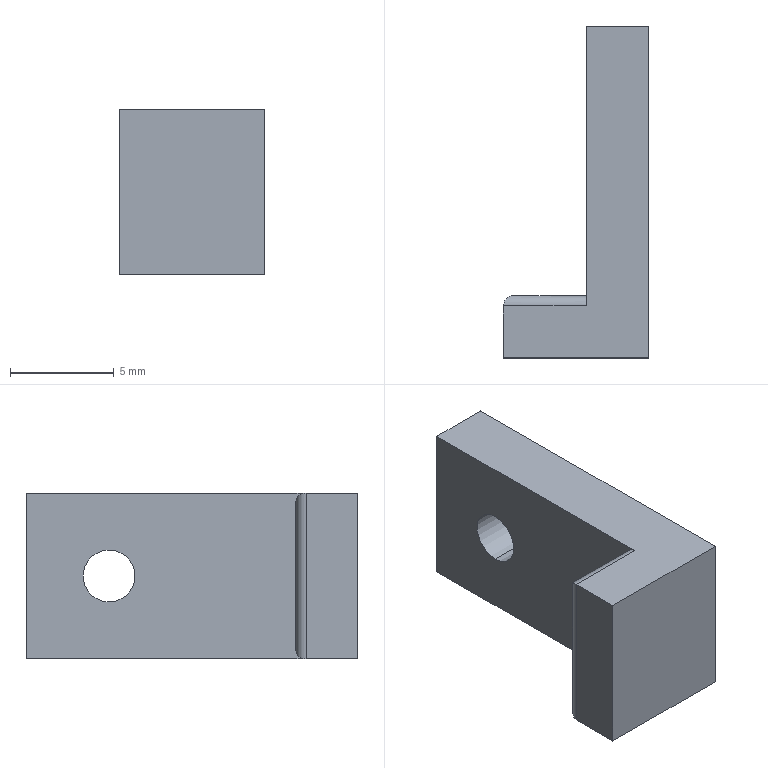Part | SolidWorks | features Extrusion 1, Fillet 1, HoleWzd 1 | 1 solid | 13 faces | box 7 x 16 x 8 mm | volume 464.439 mm3 | plane 8 | cylinder 5 | commonest cylinder face diameters 1 x3 2.5 x2
STEP:
#1=CARTESIAN_POINT('',(0.,-4.,5.25));
#2=VERTEX_POINT('',#1);
#3=CARTESIAN_POINT('',(0.,-4.,2.75));
#4=VERTEX_POINT('',#3);
#5=CARTESIAN_POINT('',(0.,-4.,4.));
#6=DIRECTION('',(1.,0.,0.));
#7=DIRECTION('',(0.,1.,0.));
#8=AXIS2_PLACEMENT_3D('',#5,#6,#7);
#9=CIRCLE('',#8,1.25);
#10=EDGE_CURVE('',#2,#4,#9,.T.);
#11=ORIENTED_EDGE('',*,*,#10,.F.);
#12=CARTESIAN_POINT('',(3.,-4.,5.25));
#13=VERTEX_POINT('',#12);
#14=CARTESIAN_POINT('',(3.,-4.,5.25));
#15=DIRECTION('',(1.,0.,0.));
#16=VECTOR('',#15,1000.);
#17=LINE('',#14,#16);
#18=EDGE_CURVE('',#2,#13,#17,.T.);
#19=ORIENTED_EDGE('',*,*,#18,.T.);
#20=CARTESIAN_POINT('',(3.,-4.,2.75));
#21=VERTEX_POINT('',#20);
#22=CARTESIAN_POINT('',(3.,-4.,4.));
#23=DIRECTION('',(1.,0.,0.));
#24=DIRECTION('',(0.,0.,-1.));
#25=AXIS2_PLACEMENT_3D('',#22,#23,#24);
#26=CIRCLE('',#25,1.25);
#27=EDGE_CURVE('',#13,#21,#26,.T.);
#28=ORIENTED_EDGE('',*,*,#27,.T.);
#29=CARTESIAN_POINT('',(3.,-4.,2.75));
#30=DIRECTION('',(1.,0.,0.));
#31=VECTOR('',#30,1000.);
#32=LINE('',#29,#31);
#33=EDGE_CURVE('',#4,#21,#32,.T.);
#34=ORIENTED_EDGE('',*,*,#33,.F.);
#35=EDGE_LOOP('',(#11,#19,#28,#34));
#36=FACE_OUTER_BOUND('',#35,.T.);
#37=CARTESIAN_POINT('',(3.,-4.,4.));
#38=DIRECTION('',(1.,0.,0.));
#39=DIRECTION('',(0.,0.,-1.));
#40=AXIS2_PLACEMENT_3D('',#37,#38,#39);
#41=CYLINDRICAL_SURFACE('',#40,1.25);
#42=ADVANCED_FACE('',(#36),#41,.F.);
#43=CARTESIAN_POINT('',(0.,-4.,4.));
#44=DIRECTION('',(1.,0.,0.));
#45=DIRECTION('',(0.,1.,0.));
#46=AXIS2_PLACEMENT_3D('',#43,#44,#45);
#47=CIRCLE('',#46,1.25);
#48=EDGE_CURVE('',#4,#2,#47,.T.);
#49=ORIENTED_EDGE('',*,*,#48,.T.);
#50=ORIENTED_EDGE('',*,*,#10,.T.);
#51=EDGE_LOOP('',(#49,#50));
#52=FACE_BOUND('',#51,.T.);
#53=CARTESIAN_POINT('',(0.,0.,0.));
#54=VERTEX_POINT('',#53);
#55=CARTESIAN_POINT('',(0.,-13.5,0.));
#56=VERTEX_POINT('',#55);
#57=CARTESIAN_POINT('',(0.,0.,0.));
#58=DIRECTION('',(0.,-1.,0.));
#59=VECTOR('',#58,1000.);
#60=LINE('',#57,#59);
#61=EDGE_CURVE('',#54,#56,#60,.T.);
#62=ORIENTED_EDGE('',*,*,#61,.T.);
#63=CARTESIAN_POINT('',(0.,-13.,0.5));
#64=VERTEX_POINT('',#63);
#65=CARTESIAN_POINT('',(0.,-13.5,0.5));
#66=DIRECTION('',(1.,0.,0.));
#67=DIRECTION('',(0.,1.,0.));
#68=AXIS2_PLACEMENT_3D('',#65,#66,#67);
#69=CIRCLE('',#68,0.5);
#70=EDGE_CURVE('',#56,#64,#69,.T.);
#71=ORIENTED_EDGE('',*,*,#70,.T.);
#72=CARTESIAN_POINT('',(0.,-13.,7.5));
#73=VERTEX_POINT('',#72);
#74=CARTESIAN_POINT('',(0.,-13.,8.));
#75=DIRECTION('',(0.,0.,-1.));
#76=VECTOR('',#75,1000.);
#77=LINE('',#74,#76);
#78=EDGE_CURVE('',#73,#64,#77,.T.);
#79=ORIENTED_EDGE('',*,*,#78,.F.);
#80=CARTESIAN_POINT('',(0.,-13.5,8.));
#81=VERTEX_POINT('',#80);
#82=CARTESIAN_POINT('',(0.,-13.5,7.5));
#83=DIRECTION('',(1.,0.,0.));
#84=DIRECTION('',(0.,1.,0.));
#85=AXIS2_PLACEMENT_3D('',#82,#83,#84);
#86=CIRCLE('',#85,0.5);
#87=EDGE_CURVE('',#73,#81,#86,.T.);
#88=ORIENTED_EDGE('',*,*,#87,.T.);
#89=CARTESIAN_POINT('',(0.,0.,8.));
#90=VERTEX_POINT('',#89);
#91=CARTESIAN_POINT('',(0.,0.,8.));
#92=DIRECTION('',(0.,-1.,0.));
#93=VECTOR('',#92,1000.);
#94=LINE('',#91,#93);
#95=EDGE_CURVE('',#90,#81,#94,.T.);
#96=ORIENTED_EDGE('',*,*,#95,.F.);
#97=CARTESIAN_POINT('',(0.,0.,8.));
#98=DIRECTION('',(0.,0.,-1.));
#99=VECTOR('',#98,1000.);
#100=LINE('',#97,#99);
#101=EDGE_CURVE('',#90,#54,#100,.T.);
#102=ORIENTED_EDGE('',*,*,#101,.T.);
#103=EDGE_LOOP('',(#62,#71,#79,#88,#96,#102));
#104=FACE_OUTER_BOUND('',#103,.T.);
#105=CARTESIAN_POINT('',(0.,0.,8.));
#106=DIRECTION('',(1.,0.,0.));
#107=DIRECTION('',(0.,1.,0.));
#108=AXIS2_PLACEMENT_3D('',#105,#106,#107);
#109=PLANE('',#108);
#110=ADVANCED_FACE('',(#52,#104),#109,.F.);
#111=ORIENTED_EDGE('',*,*,#78,.T.);
#112=CARTESIAN_POINT('',(-3.5,-13.,0.5));
#113=VERTEX_POINT('',#112);
#114=CARTESIAN_POINT('',(-4.,-13.,0.5));
#115=DIRECTION('',(-1.,0.,0.));
#116=VECTOR('',#115,1000.);
#117=LINE('',#114,#116);
#118=EDGE_CURVE('',#64,#113,#117,.T.);
#119=ORIENTED_EDGE('',*,*,#118,.T.);
#120=CARTESIAN_POINT('',(-3.5,-13.,7.5));
#121=VERTEX_POINT('',#120);
#122=CARTESIAN_POINT('',(-3.5,-13.,8.));
#123=DIRECTION('',(0.,0.,1.));
#124=VECTOR('',#123,1000.);
#125=LINE('',#122,#124);
#126=EDGE_CURVE('',#113,#121,#125,.T.);
#127=ORIENTED_EDGE('',*,*,#126,.T.);
#128=CARTESIAN_POINT('',(0.,-13.,7.5));
#129=DIRECTION('',(1.,0.,0.));
#130=VECTOR('',#129,1000.);
#131=LINE('',#128,#130);
#132=EDGE_CURVE('',#121,#73,#131,.T.);
#133=ORIENTED_EDGE('',*,*,#132,.T.);
#134=EDGE_LOOP('',(#111,#119,#127,#133));
#135=FACE_OUTER_BOUND('',#134,.T.);
#136=CARTESIAN_POINT('',(0.,-13.,8.));
#137=DIRECTION('',(0.,-1.,0.));
#138=DIRECTION('',(0.,0.,-1.));
#139=AXIS2_PLACEMENT_3D('',#136,#137,#138);
#140=PLANE('',#139);
#141=ADVANCED_FACE('',(#135),#140,.F.);
#142=CARTESIAN_POINT('',(-4.,-13.5,8.));
#143=VERTEX_POINT('',#142);
#144=CARTESIAN_POINT('',(-4.,-16.,8.));
#145=VERTEX_POINT('',#144);
#146=CARTESIAN_POINT('',(-4.,-16.,8.));
#147=DIRECTION('',(0.,-1.,0.));
#148=VECTOR('',#147,1000.);
#149=LINE('',#146,#148);
#150=EDGE_CURVE('',#143,#145,#149,.T.);
#151=ORIENTED_EDGE('',*,*,#150,.F.);
#152=CARTESIAN_POINT('',(-4.,-13.5,0.));
#153=VERTEX_POINT('',#152);
#154=CARTESIAN_POINT('',(-4.,-13.5,8.));
#155=DIRECTION('',(0.,0.,-1.));
#156=VECTOR('',#155,1000.);
#157=LINE('',#154,#156);
#158=EDGE_CURVE('',#143,#153,#157,.T.);
#159=ORIENTED_EDGE('',*,*,#158,.T.);
#160=CARTESIAN_POINT('',(-4.,-16.,0.));
#161=VERTEX_POINT('',#160);
#162=CARTESIAN_POINT('',(-4.,-16.,0.));
#163=DIRECTION('',(0.,-1.,0.));
#164=VECTOR('',#163,1000.);
#165=LINE('',#162,#164);
#166=EDGE_CURVE('',#153,#161,#165,.T.);
#167=ORIENTED_EDGE('',*,*,#166,.T.);
#168=CARTESIAN_POINT('',(-4.,-16.,8.));
#169=DIRECTION('',(0.,0.,-1.));
#170=VECTOR('',#169,1000.);
#171=LINE('',#168,#170);
#172=EDGE_CURVE('',#145,#161,#171,.T.);
#173=ORIENTED_EDGE('',*,*,#172,.F.);
#174=EDGE_LOOP('',(#151,#159,#167,#173));
#175=FACE_OUTER_BOUND('',#174,.T.);
#176=CARTESIAN_POINT('',(-4.,-16.,8.));
#177=DIRECTION('',(1.,0.,0.));
#178=DIRECTION('',(0.,0.,-1.));
#179=AXIS2_PLACEMENT_3D('',#176,#177,#178);
#180=PLANE('',#179);
#181=ADVANCED_FACE('',(#175),#180,.F.);
#182=CARTESIAN_POINT('',(3.,-16.,0.));
#183=VERTEX_POINT('',#182);
#184=CARTESIAN_POINT('',(-4.,-16.,0.));
#185=DIRECTION('',(1.,0.,0.));
#186=VECTOR('',#185,1000.);
#187=LINE('',#184,#186);
#188=EDGE_CURVE('',#161,#183,#187,.T.);
#189=ORIENTED_EDGE('',*,*,#188,.T.);
#190=CARTESIAN_POINT('',(3.,-16.,8.));
#191=VERTEX_POINT('',#190);
#192=CARTESIAN_POINT('',(3.,-16.,8.));
#193=DIRECTION('',(0.,0.,-1.));
#194=VECTOR('',#193,1000.);
#195=LINE('',#192,#194);
#196=EDGE_CURVE('',#191,#183,#195,.T.);
#197=ORIENTED_EDGE('',*,*,#196,.F.);
#198=CARTESIAN_POINT('',(-4.,-16.,8.));
#199=DIRECTION('',(1.,0.,0.));
#200=VECTOR('',#199,1000.);
#201=LINE('',#198,#200);
#202=EDGE_CURVE('',#145,#191,#201,.T.);
#203=ORIENTED_EDGE('',*,*,#202,.F.);
#204=ORIENTED_EDGE('',*,*,#172,.T.);
#205=EDGE_LOOP('',(#189,#197,#203,#204));
#206=FACE_OUTER_BOUND('',#205,.T.);
#207=CARTESIAN_POINT('',(-4.,-16.,8.));
#208=DIRECTION('',(0.,1.,0.));
#209=DIRECTION('',(0.,0.,1.));
#210=AXIS2_PLACEMENT_3D('',#207,#208,#209);
#211=PLANE('',#210);
#212=ADVANCED_FACE('',(#206),#211,.F.);
#213=CARTESIAN_POINT('',(3.,-4.,4.));
#214=DIRECTION('',(1.,0.,0.));
#215=DIRECTION('',(0.,0.,-1.));
#216=AXIS2_PLACEMENT_3D('',#213,#214,#215);
#217=CIRCLE('',#216,1.25);
#218=EDGE_CURVE('',#21,#13,#217,.T.);
#219=ORIENTED_EDGE('',*,*,#218,.F.);
#220=ORIENTED_EDGE('',*,*,#27,.F.);
#221=EDGE_LOOP('',(#219,#220));
#222=FACE_BOUND('',#221,.T.);
#223=CARTESIAN_POINT('',(3.,0.,0.));
#224=VERTEX_POINT('',#223);
#225=CARTESIAN_POINT('',(3.,0.,0.));
#226=DIRECTION('',(0.,1.,0.));
#227=VECTOR('',#226,1000.);
#228=LINE('',#225,#227);
#229=EDGE_CURVE('',#183,#224,#228,.T.);
#230=ORIENTED_EDGE('',*,*,#229,.T.);
#231=CARTESIAN_POINT('',(3.,0.,8.));
#232=VERTEX_POINT('',#231);
#233=CARTESIAN_POINT('',(3.,0.,8.));
#234=DIRECTION('',(0.,0.,-1.));
#235=VECTOR('',#234,1000.);
#236=LINE('',#233,#235);
#237=EDGE_CURVE('',#232,#224,#236,.T.);
#238=ORIENTED_EDGE('',*,*,#237,.F.);
#239=CARTESIAN_POINT('',(3.,0.,8.));
#240=DIRECTION('',(0.,1.,0.));
#241=VECTOR('',#240,1000.);
#242=LINE('',#239,#241);
#243=EDGE_CURVE('',#191,#232,#242,.T.);
#244=ORIENTED_EDGE('',*,*,#243,.F.);
#245=ORIENTED_EDGE('',*,*,#196,.T.);
#246=EDGE_LOOP('',(#230,#238,#244,#245));
#247=FACE_OUTER_BOUND('',#246,.T.);
#248=CARTESIAN_POINT('',(3.,0.,8.));
#249=DIRECTION('',(-1.,0.,0.));
#250=DIRECTION('',(0.,-1.,0.));
#251=AXIS2_PLACEMENT_3D('',#248,#249,#250);
#252=PLANE('',#251);
#253=ADVANCED_FACE('',(#222,#247),#252,.F.);
#254=CARTESIAN_POINT('',(0.,0.,0.));
#255=DIRECTION('',(-1.,0.,0.));
#256=VECTOR('',#255,1000.);
#257=LINE('',#254,#256);
#258=EDGE_CURVE('',#224,#54,#257,.T.);
#259=ORIENTED_EDGE('',*,*,#258,.T.);
#260=ORIENTED_EDGE('',*,*,#101,.F.);
#261=CARTESIAN_POINT('',(0.,0.,8.));
#262=DIRECTION('',(-1.,0.,0.));
#263=VECTOR('',#262,1000.);
#264=LINE('',#261,#263);
#265=EDGE_CURVE('',#232,#90,#264,.T.);
#266=ORIENTED_EDGE('',*,*,#265,.F.);
#267=ORIENTED_EDGE('',*,*,#237,.T.);
#268=EDGE_LOOP('',(#259,#260,#266,#267));
#269=FACE_OUTER_BOUND('',#268,.T.);
#270=CARTESIAN_POINT('',(0.,0.,8.));
#271=DIRECTION('',(0.,-1.,0.));
#272=DIRECTION('',(0.,0.,-1.));
#273=AXIS2_PLACEMENT_3D('',#270,#271,#272);
#274=PLANE('',#273);
#275=ADVANCED_FACE('',(#269),#274,.F.);
#276=ORIENTED_EDGE('',*,*,#95,.T.);
#277=CARTESIAN_POINT('',(0.,-13.5,8.));
#278=DIRECTION('',(-1.,0.,0.));
#279=VECTOR('',#278,1000.);
#280=LINE('',#277,#279);
#281=EDGE_CURVE('',#81,#143,#280,.T.);
#282=ORIENTED_EDGE('',*,*,#281,.T.);
#283=ORIENTED_EDGE('',*,*,#150,.T.);
#284=ORIENTED_EDGE('',*,*,#202,.T.);
#285=ORIENTED_EDGE('',*,*,#243,.T.);
#286=ORIENTED_EDGE('',*,*,#265,.T.);
#287=EDGE_LOOP('',(#276,#282,#283,#284,#285,#286));
#288=FACE_OUTER_BOUND('',#287,.T.);
#289=CARTESIAN_POINT('',(0.,0.,8.));
#290=DIRECTION('',(0.,0.,-1.));
#291=DIRECTION('',(-1.,0.,0.));
#292=AXIS2_PLACEMENT_3D('',#289,#290,#291);
#293=PLANE('',#292);
#294=ADVANCED_FACE('',(#288),#293,.F.);
#295=ORIENTED_EDGE('',*,*,#166,.F.);
#296=CARTESIAN_POINT('',(0.,-13.5,0.));
#297=DIRECTION('',(1.,0.,0.));
#298=VECTOR('',#297,1000.);
#299=LINE('',#296,#298);
#300=EDGE_CURVE('',#153,#56,#299,.T.);
#301=ORIENTED_EDGE('',*,*,#300,.T.);
#302=ORIENTED_EDGE('',*,*,#61,.F.);
#303=ORIENTED_EDGE('',*,*,#258,.F.);
#304=ORIENTED_EDGE('',*,*,#229,.F.);
#305=ORIENTED_EDGE('',*,*,#188,.F.);
#306=EDGE_LOOP('',(#295,#301,#302,#303,#304,#305));
#307=FACE_OUTER_BOUND('',#306,.T.);
#308=CARTESIAN_POINT('',(0.,0.,0.));
#309=DIRECTION('',(0.,0.,-1.));
#310=DIRECTION('',(-1.,0.,0.));
#311=AXIS2_PLACEMENT_3D('',#308,#309,#310);
#312=PLANE('',#311);
#313=ADVANCED_FACE('',(#307),#312,.T.);
#314=ORIENTED_EDGE('',*,*,#18,.F.);
#315=ORIENTED_EDGE('',*,*,#48,.F.);
#316=ORIENTED_EDGE('',*,*,#33,.T.);
#317=ORIENTED_EDGE('',*,*,#218,.T.);
#318=EDGE_LOOP('',(#314,#315,#316,#317));
#319=FACE_OUTER_BOUND('',#318,.T.);
#320=CARTESIAN_POINT('',(3.,-4.,4.));
#321=DIRECTION('',(1.,0.,0.));
#322=DIRECTION('',(0.,0.,-1.));
#323=AXIS2_PLACEMENT_3D('',#320,#321,#322);
#324=CYLINDRICAL_SURFACE('',#323,1.25);
#325=ADVANCED_FACE('',(#319),#324,.F.);
#326=ORIENTED_EDGE('',*,*,#87,.F.);
#327=ORIENTED_EDGE('',*,*,#132,.F.);
#328=CARTESIAN_POINT('',(-4.,-13.5,8.));
#329=CARTESIAN_POINT('',(-4.,-13.207,8.));
#330=CARTESIAN_POINT('',(-3.793,-13.,7.793));
#331=CARTESIAN_POINT('',(-3.5,-13.,7.5));
#332=(BOUNDED_CURVE()B_SPLINE_CURVE(3,(#328,#329,#330,#331),.UNSPECIFIED.,.F.,.F.)B_SPLINE_CURVE_WITH_KNOTS((4,4),(0.,1.571),.UNSPECIFIED.)CURVE()GEOMETRIC_REPRESENTATION_ITEM()RATIONAL_B_SPLINE_CURVE((1.,0.8047,0.8047,1.))REPRESENTATION_ITEM(''));
#333=EDGE_CURVE('',#143,#121,#332,.T.);
#334=ORIENTED_EDGE('',*,*,#333,.F.);
#335=ORIENTED_EDGE('',*,*,#281,.F.);
#336=EDGE_LOOP('',(#326,#327,#334,#335));
#337=FACE_OUTER_BOUND('',#336,.T.);
#338=CARTESIAN_POINT('',(0.,-13.5,7.5));
#339=DIRECTION('',(-1.,0.,0.));
#340=DIRECTION('',(0.,0.,1.));
#341=AXIS2_PLACEMENT_3D('',#338,#339,#340);
#342=CYLINDRICAL_SURFACE('',#341,0.5);
#343=ADVANCED_FACE('',(#337),#342,.T.);
#344=ORIENTED_EDGE('',*,*,#333,.T.);
#345=ORIENTED_EDGE('',*,*,#126,.F.);
#346=CARTESIAN_POINT('',(-4.,-13.5,0.));
#347=CARTESIAN_POINT('',(-4.,-13.207,0.));
#348=CARTESIAN_POINT('',(-3.793,-13.,0.2071));
#349=CARTESIAN_POINT('',(-3.5,-13.,0.5));
#350=(BOUNDED_CURVE()B_SPLINE_CURVE(3,(#346,#347,#348,#349),.UNSPECIFIED.,.F.,.F.)B_SPLINE_CURVE_WITH_KNOTS((4,4),(0.,1.571),.UNSPECIFIED.)CURVE()GEOMETRIC_REPRESENTATION_ITEM()RATIONAL_B_SPLINE_CURVE((1.,0.8047,0.8047,1.))REPRESENTATION_ITEM(''));
#351=EDGE_CURVE('',#153,#113,#350,.T.);
#352=ORIENTED_EDGE('',*,*,#351,.F.);
#353=ORIENTED_EDGE('',*,*,#158,.F.);
#354=EDGE_LOOP('',(#344,#345,#352,#353));
#355=FACE_OUTER_BOUND('',#354,.T.);
#356=CARTESIAN_POINT('',(-3.5,-13.5,8.));
#357=DIRECTION('',(0.,0.,-1.));
#358=DIRECTION('',(-1.,0.,0.));
#359=AXIS2_PLACEMENT_3D('',#356,#357,#358);
#360=CYLINDRICAL_SURFACE('',#359,0.5);
#361=ADVANCED_FACE('',(#355),#360,.T.);
#362=ORIENTED_EDGE('',*,*,#70,.F.);
#363=ORIENTED_EDGE('',*,*,#300,.F.);
#364=ORIENTED_EDGE('',*,*,#351,.T.);
#365=ORIENTED_EDGE('',*,*,#118,.F.);
#366=EDGE_LOOP('',(#362,#363,#364,#365));
#367=FACE_OUTER_BOUND('',#366,.T.);
#368=CARTESIAN_POINT('',(0.,-13.5,0.5));
#369=DIRECTION('',(1.,0.,0.));
#370=DIRECTION('',(0.,0.,-1.));
#371=AXIS2_PLACEMENT_3D('',#368,#369,#370);
#372=CYLINDRICAL_SURFACE('',#371,0.5);
#373=ADVANCED_FACE('',(#367),#372,.T.);
#374=CLOSED_SHELL('',(#42,#110,#141,#181,#212,#253,#275,#294,#313,#325,#343,#361,#373));
#375=MANIFOLD_SOLID_BREP('',#374);
#376=CARTESIAN_POINT('',(0.,0.,0.));
#377=DIRECTION('',(0.,0.,1.));
#378=DIRECTION('',(1.,0.,0.));
#379=AXIS2_PLACEMENT_3D('',#376,#377,#378);
#380=(LENGTH_UNIT()NAMED_UNIT(*)SI_UNIT(.MILLI.,.METRE.));
#381=UNCERTAINTY_MEASURE_WITH_UNIT(LENGTH_MEASURE(0.00001),#380,'','');
#382=(NAMED_UNIT(*)PLANE_ANGLE_UNIT()SI_UNIT($,.RADIAN.));
#383=(NAMED_UNIT(*)SI_UNIT($,.STERADIAN.)SOLID_ANGLE_UNIT());
#384=(GEOMETRIC_REPRESENTATION_CONTEXT(3)GLOBAL_UNCERTAINTY_ASSIGNED_CONTEXT((#381))GLOBAL_UNIT_ASSIGNED_CONTEXT((#380,#382,#383))REPRESENTATION_CONTEXT('',''));
#385=ADVANCED_BREP_SHAPE_REPRESENTATION('',(#375,#379),#384);